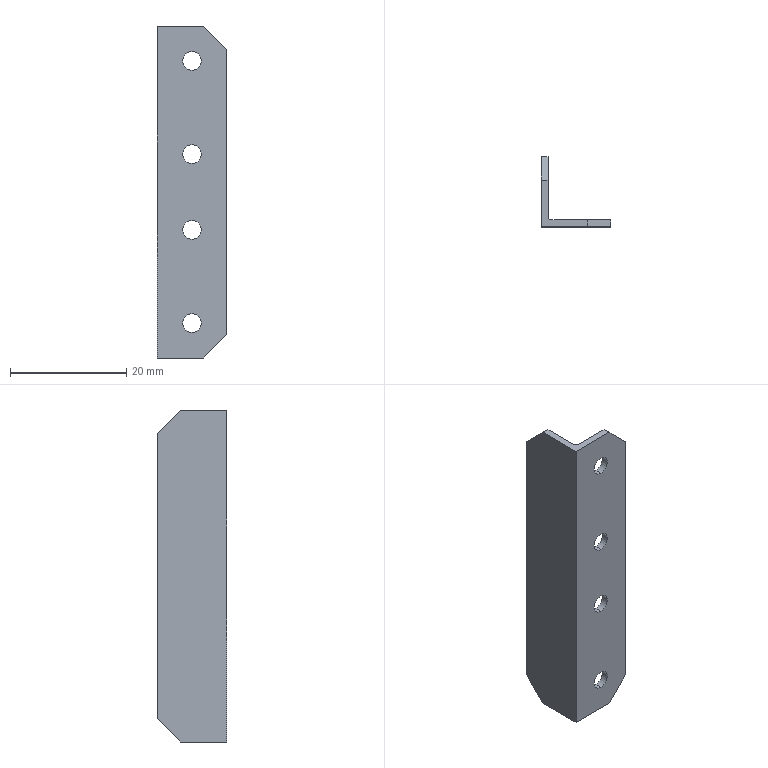Part | SolidWorks | features BaseBody 1 | 1 solid | 21 faces | box 12 x 12 x 57 mm | volume 1486 mm3 | plane 12 | cylinder 9 | commonest cylinder face diameters 3.2 x8 1 x1
STEP:
#1=CARTESIAN_POINT('',(6.,1.2,33.4));
#2=VERTEX_POINT('',#1);
#3=CARTESIAN_POINT('',(6.,1.2,36.6));
#4=VERTEX_POINT('',#3);
#5=CARTESIAN_POINT('',(6.,1.2,35.));
#6=DIRECTION('',(0.,1.,0.));
#7=DIRECTION('',(0.,0.,-1.));
#8=AXIS2_PLACEMENT_3D('',#5,#6,#7);
#9=CIRCLE('',#8,1.6);
#10=EDGE_CURVE('',#2,#4,#9,.T.);
#11=ORIENTED_EDGE('',*,*,#10,.T.);
#12=CARTESIAN_POINT('',(6.,0.,36.6));
#13=VERTEX_POINT('',#12);
#14=CARTESIAN_POINT('',(6.,1.2,36.6));
#15=DIRECTION('',(0.,-1.,0.));
#16=VECTOR('',#15,1000.);
#17=LINE('',#14,#16);
#18=EDGE_CURVE('',#4,#13,#17,.T.);
#19=ORIENTED_EDGE('',*,*,#18,.T.);
#20=CARTESIAN_POINT('',(6.,0.,33.4));
#21=VERTEX_POINT('',#20);
#22=CARTESIAN_POINT('',(6.,0.,35.));
#23=DIRECTION('',(0.,-1.,0.));
#24=DIRECTION('',(0.,0.,-1.));
#25=AXIS2_PLACEMENT_3D('',#22,#23,#24);
#26=CIRCLE('',#25,1.6);
#27=EDGE_CURVE('',#13,#21,#26,.T.);
#28=ORIENTED_EDGE('',*,*,#27,.T.);
#29=CARTESIAN_POINT('',(6.,1.2,33.4));
#30=DIRECTION('',(0.,-1.,0.));
#31=VECTOR('',#30,1000.);
#32=LINE('',#29,#31);
#33=EDGE_CURVE('',#2,#21,#32,.T.);
#34=ORIENTED_EDGE('',*,*,#33,.F.);
#35=EDGE_LOOP('',(#11,#19,#28,#34));
#36=FACE_OUTER_BOUND('',#35,.T.);
#37=CARTESIAN_POINT('',(6.,1.2,35.));
#38=DIRECTION('',(0.,-1.,0.));
#39=DIRECTION('',(0.,0.,-1.));
#40=AXIS2_PLACEMENT_3D('',#37,#38,#39);
#41=CYLINDRICAL_SURFACE('',#40,1.6);
#42=ADVANCED_FACE('',(#36),#41,.F.);
#43=CARTESIAN_POINT('',(6.,1.2,4.4));
#44=VERTEX_POINT('',#43);
#45=CARTESIAN_POINT('',(6.,1.2,7.6));
#46=VERTEX_POINT('',#45);
#47=CARTESIAN_POINT('',(6.,1.2,6.));
#48=DIRECTION('',(0.,1.,0.));
#49=DIRECTION('',(0.,0.,-1.));
#50=AXIS2_PLACEMENT_3D('',#47,#48,#49);
#51=CIRCLE('',#50,1.6);
#52=EDGE_CURVE('',#44,#46,#51,.T.);
#53=ORIENTED_EDGE('',*,*,#52,.T.);
#54=CARTESIAN_POINT('',(6.,0.,7.6));
#55=VERTEX_POINT('',#54);
#56=CARTESIAN_POINT('',(6.,1.2,7.6));
#57=DIRECTION('',(0.,-1.,0.));
#58=VECTOR('',#57,1000.);
#59=LINE('',#56,#58);
#60=EDGE_CURVE('',#46,#55,#59,.T.);
#61=ORIENTED_EDGE('',*,*,#60,.T.);
#62=CARTESIAN_POINT('',(6.,0.,4.4));
#63=VERTEX_POINT('',#62);
#64=CARTESIAN_POINT('',(6.,0.,6.));
#65=DIRECTION('',(0.,-1.,0.));
#66=DIRECTION('',(0.,0.,-1.));
#67=AXIS2_PLACEMENT_3D('',#64,#65,#66);
#68=CIRCLE('',#67,1.6);
#69=EDGE_CURVE('',#55,#63,#68,.T.);
#70=ORIENTED_EDGE('',*,*,#69,.T.);
#71=CARTESIAN_POINT('',(6.,1.2,4.4));
#72=DIRECTION('',(0.,-1.,0.));
#73=VECTOR('',#72,1000.);
#74=LINE('',#71,#73);
#75=EDGE_CURVE('',#44,#63,#74,.T.);
#76=ORIENTED_EDGE('',*,*,#75,.F.);
#77=EDGE_LOOP('',(#53,#61,#70,#76));
#78=FACE_OUTER_BOUND('',#77,.T.);
#79=CARTESIAN_POINT('',(6.,1.2,6.));
#80=DIRECTION('',(0.,-1.,0.));
#81=DIRECTION('',(0.,0.,-1.));
#82=AXIS2_PLACEMENT_3D('',#79,#80,#81);
#83=CYLINDRICAL_SURFACE('',#82,1.6);
#84=ADVANCED_FACE('',(#78),#83,.F.);
#85=CARTESIAN_POINT('',(6.,1.2,49.4));
#86=VERTEX_POINT('',#85);
#87=CARTESIAN_POINT('',(6.,1.2,52.6));
#88=VERTEX_POINT('',#87);
#89=CARTESIAN_POINT('',(6.,1.2,51.));
#90=DIRECTION('',(0.,1.,0.));
#91=DIRECTION('',(0.,0.,-1.));
#92=AXIS2_PLACEMENT_3D('',#89,#90,#91);
#93=CIRCLE('',#92,1.6);
#94=EDGE_CURVE('',#86,#88,#93,.T.);
#95=ORIENTED_EDGE('',*,*,#94,.T.);
#96=CARTESIAN_POINT('',(6.,0.,52.6));
#97=VERTEX_POINT('',#96);
#98=CARTESIAN_POINT('',(6.,1.2,52.6));
#99=DIRECTION('',(0.,-1.,0.));
#100=VECTOR('',#99,1000.);
#101=LINE('',#98,#100);
#102=EDGE_CURVE('',#88,#97,#101,.T.);
#103=ORIENTED_EDGE('',*,*,#102,.T.);
#104=CARTESIAN_POINT('',(6.,0.,49.4));
#105=VERTEX_POINT('',#104);
#106=CARTESIAN_POINT('',(6.,0.,51.));
#107=DIRECTION('',(0.,-1.,0.));
#108=DIRECTION('',(0.,0.,-1.));
#109=AXIS2_PLACEMENT_3D('',#106,#107,#108);
#110=CIRCLE('',#109,1.6);
#111=EDGE_CURVE('',#97,#105,#110,.T.);
#112=ORIENTED_EDGE('',*,*,#111,.T.);
#113=CARTESIAN_POINT('',(6.,1.2,49.4));
#114=DIRECTION('',(0.,-1.,0.));
#115=VECTOR('',#114,1000.);
#116=LINE('',#113,#115);
#117=EDGE_CURVE('',#86,#105,#116,.T.);
#118=ORIENTED_EDGE('',*,*,#117,.F.);
#119=EDGE_LOOP('',(#95,#103,#112,#118));
#120=FACE_OUTER_BOUND('',#119,.T.);
#121=CARTESIAN_POINT('',(6.,1.2,51.));
#122=DIRECTION('',(0.,-1.,0.));
#123=DIRECTION('',(0.,0.,-1.));
#124=AXIS2_PLACEMENT_3D('',#121,#122,#123);
#125=CYLINDRICAL_SURFACE('',#124,1.6);
#126=ADVANCED_FACE('',(#120),#125,.F.);
#127=CARTESIAN_POINT('',(6.,1.2,20.4));
#128=VERTEX_POINT('',#127);
#129=CARTESIAN_POINT('',(6.,1.2,23.6));
#130=VERTEX_POINT('',#129);
#131=CARTESIAN_POINT('',(6.,1.2,22.));
#132=DIRECTION('',(0.,1.,0.));
#133=DIRECTION('',(0.,0.,-1.));
#134=AXIS2_PLACEMENT_3D('',#131,#132,#133);
#135=CIRCLE('',#134,1.6);
#136=EDGE_CURVE('',#128,#130,#135,.T.);
#137=ORIENTED_EDGE('',*,*,#136,.T.);
#138=CARTESIAN_POINT('',(6.,0.,23.6));
#139=VERTEX_POINT('',#138);
#140=CARTESIAN_POINT('',(6.,1.2,23.6));
#141=DIRECTION('',(0.,-1.,0.));
#142=VECTOR('',#141,1000.);
#143=LINE('',#140,#142);
#144=EDGE_CURVE('',#130,#139,#143,.T.);
#145=ORIENTED_EDGE('',*,*,#144,.T.);
#146=CARTESIAN_POINT('',(6.,0.,20.4));
#147=VERTEX_POINT('',#146);
#148=CARTESIAN_POINT('',(6.,0.,22.));
#149=DIRECTION('',(0.,-1.,0.));
#150=DIRECTION('',(0.,0.,-1.));
#151=AXIS2_PLACEMENT_3D('',#148,#149,#150);
#152=CIRCLE('',#151,1.6);
#153=EDGE_CURVE('',#139,#147,#152,.T.);
#154=ORIENTED_EDGE('',*,*,#153,.T.);
#155=CARTESIAN_POINT('',(6.,1.2,20.4));
#156=DIRECTION('',(0.,-1.,0.));
#157=VECTOR('',#156,1000.);
#158=LINE('',#155,#157);
#159=EDGE_CURVE('',#128,#147,#158,.T.);
#160=ORIENTED_EDGE('',*,*,#159,.F.);
#161=EDGE_LOOP('',(#137,#145,#154,#160));
#162=FACE_OUTER_BOUND('',#161,.T.);
#163=CARTESIAN_POINT('',(6.,1.2,22.));
#164=DIRECTION('',(0.,-1.,0.));
#165=DIRECTION('',(0.,0.,-1.));
#166=AXIS2_PLACEMENT_3D('',#163,#164,#165);
#167=CYLINDRICAL_SURFACE('',#166,1.6);
#168=ADVANCED_FACE('',(#162),#167,.F.);
#169=ORIENTED_EDGE('',*,*,#18,.F.);
#170=CARTESIAN_POINT('',(6.,1.2,35.));
#171=DIRECTION('',(0.,1.,0.));
#172=DIRECTION('',(0.,0.,-1.));
#173=AXIS2_PLACEMENT_3D('',#170,#171,#172);
#174=CIRCLE('',#173,1.6);
#175=EDGE_CURVE('',#4,#2,#174,.T.);
#176=ORIENTED_EDGE('',*,*,#175,.T.);
#177=ORIENTED_EDGE('',*,*,#33,.T.);
#178=CARTESIAN_POINT('',(6.,0.,35.));
#179=DIRECTION('',(0.,-1.,0.));
#180=DIRECTION('',(0.,0.,-1.));
#181=AXIS2_PLACEMENT_3D('',#178,#179,#180);
#182=CIRCLE('',#181,1.6);
#183=EDGE_CURVE('',#21,#13,#182,.T.);
#184=ORIENTED_EDGE('',*,*,#183,.T.);
#185=EDGE_LOOP('',(#169,#176,#177,#184));
#186=FACE_OUTER_BOUND('',#185,.T.);
#187=CARTESIAN_POINT('',(6.,1.2,35.));
#188=DIRECTION('',(0.,-1.,0.));
#189=DIRECTION('',(0.,0.,-1.));
#190=AXIS2_PLACEMENT_3D('',#187,#188,#189);
#191=CYLINDRICAL_SURFACE('',#190,1.6);
#192=ADVANCED_FACE('',(#186),#191,.F.);
#193=CARTESIAN_POINT('',(6.,0.,6.));
#194=DIRECTION('',(0.,-1.,0.));
#195=DIRECTION('',(0.,0.,-1.));
#196=AXIS2_PLACEMENT_3D('',#193,#194,#195);
#197=CIRCLE('',#196,1.6);
#198=EDGE_CURVE('',#63,#55,#197,.T.);
#199=ORIENTED_EDGE('',*,*,#198,.F.);
#200=ORIENTED_EDGE('',*,*,#69,.F.);
#201=EDGE_LOOP('',(#199,#200));
#202=FACE_BOUND('',#201,.T.);
#203=CARTESIAN_POINT('',(6.,0.,51.));
#204=DIRECTION('',(0.,-1.,0.));
#205=DIRECTION('',(0.,0.,-1.));
#206=AXIS2_PLACEMENT_3D('',#203,#204,#205);
#207=CIRCLE('',#206,1.6);
#208=EDGE_CURVE('',#105,#97,#207,.T.);
#209=ORIENTED_EDGE('',*,*,#208,.F.);
#210=ORIENTED_EDGE('',*,*,#111,.F.);
#211=EDGE_LOOP('',(#209,#210));
#212=FACE_BOUND('',#211,.T.);
#213=CARTESIAN_POINT('',(6.,0.,22.));
#214=DIRECTION('',(0.,-1.,0.));
#215=DIRECTION('',(0.,0.,-1.));
#216=AXIS2_PLACEMENT_3D('',#213,#214,#215);
#217=CIRCLE('',#216,1.6);
#218=EDGE_CURVE('',#147,#139,#217,.T.);
#219=ORIENTED_EDGE('',*,*,#218,.F.);
#220=ORIENTED_EDGE('',*,*,#153,.F.);
#221=EDGE_LOOP('',(#219,#220));
#222=FACE_BOUND('',#221,.T.);
#223=ORIENTED_EDGE('',*,*,#183,.F.);
#224=ORIENTED_EDGE('',*,*,#27,.F.);
#225=EDGE_LOOP('',(#223,#224));
#226=FACE_BOUND('',#225,.T.);
#227=CARTESIAN_POINT('',(8.,0.,57.));
#228=VERTEX_POINT('',#227);
#229=CARTESIAN_POINT('',(12.,0.,53.));
#230=VERTEX_POINT('',#229);
#231=CARTESIAN_POINT('',(8.,0.,57.));
#232=DIRECTION('',(0.7071,0.,-0.7071));
#233=VECTOR('',#232,1000.);
#234=LINE('',#231,#233);
#235=EDGE_CURVE('',#228,#230,#234,.T.);
#236=ORIENTED_EDGE('',*,*,#235,.F.);
#237=CARTESIAN_POINT('',(0.,0.,57.));
#238=VERTEX_POINT('',#237);
#239=CARTESIAN_POINT('',(6.,0.,57.));
#240=DIRECTION('',(1.,0.,0.));
#241=VECTOR('',#240,1000.);
#242=LINE('',#239,#241);
#243=EDGE_CURVE('',#238,#228,#242,.T.);
#244=ORIENTED_EDGE('',*,*,#243,.F.);
#245=CARTESIAN_POINT('',(0.,0.,0.));
#246=VERTEX_POINT('',#245);
#247=CARTESIAN_POINT('',(0.,0.,28.5));
#248=DIRECTION('',(0.,0.,1.));
#249=VECTOR('',#248,1000.);
#250=LINE('',#247,#249);
#251=EDGE_CURVE('',#246,#238,#250,.T.);
#252=ORIENTED_EDGE('',*,*,#251,.F.);
#253=CARTESIAN_POINT('',(8.,0.,0.));
#254=VERTEX_POINT('',#253);
#255=CARTESIAN_POINT('',(6.,0.,0.));
#256=DIRECTION('',(-1.,0.,0.));
#257=VECTOR('',#256,1000.);
#258=LINE('',#255,#257);
#259=EDGE_CURVE('',#254,#246,#258,.T.);
#260=ORIENTED_EDGE('',*,*,#259,.F.);
#261=CARTESIAN_POINT('',(12.,0.,4.));
#262=VERTEX_POINT('',#261);
#263=CARTESIAN_POINT('',(8.,0.,0.));
#264=DIRECTION('',(-0.7071,0.,-0.7071));
#265=VECTOR('',#264,1000.);
#266=LINE('',#263,#265);
#267=EDGE_CURVE('',#262,#254,#266,.T.);
#268=ORIENTED_EDGE('',*,*,#267,.F.);
#269=CARTESIAN_POINT('',(12.,0.,28.5));
#270=DIRECTION('',(0.,0.,-1.));
#271=VECTOR('',#270,1000.);
#272=LINE('',#269,#271);
#273=EDGE_CURVE('',#230,#262,#272,.T.);
#274=ORIENTED_EDGE('',*,*,#273,.F.);
#275=EDGE_LOOP('',(#236,#244,#252,#260,#268,#274));
#276=FACE_OUTER_BOUND('',#275,.T.);
#277=CARTESIAN_POINT('',(0.,0.,0.));
#278=DIRECTION('',(0.,1.,0.));
#279=DIRECTION('',(0.,0.,1.));
#280=AXIS2_PLACEMENT_3D('',#277,#278,#279);
#281=PLANE('',#280);
#282=ADVANCED_FACE('',(#202,#212,#222,#226,#276),#281,.F.);
#283=ORIENTED_EDGE('',*,*,#52,.F.);
#284=CARTESIAN_POINT('',(6.,1.2,6.));
#285=DIRECTION('',(0.,1.,0.));
#286=DIRECTION('',(0.,0.,-1.));
#287=AXIS2_PLACEMENT_3D('',#284,#285,#286);
#288=CIRCLE('',#287,1.6);
#289=EDGE_CURVE('',#46,#44,#288,.T.);
#290=ORIENTED_EDGE('',*,*,#289,.F.);
#291=EDGE_LOOP('',(#283,#290));
#292=FACE_BOUND('',#291,.T.);
#293=ORIENTED_EDGE('',*,*,#94,.F.);
#294=CARTESIAN_POINT('',(6.,1.2,51.));
#295=DIRECTION('',(0.,1.,0.));
#296=DIRECTION('',(0.,0.,-1.));
#297=AXIS2_PLACEMENT_3D('',#294,#295,#296);
#298=CIRCLE('',#297,1.6);
#299=EDGE_CURVE('',#88,#86,#298,.T.);
#300=ORIENTED_EDGE('',*,*,#299,.F.);
#301=EDGE_LOOP('',(#293,#300));
#302=FACE_BOUND('',#301,.T.);
#303=ORIENTED_EDGE('',*,*,#136,.F.);
#304=CARTESIAN_POINT('',(6.,1.2,22.));
#305=DIRECTION('',(0.,1.,0.));
#306=DIRECTION('',(0.,0.,-1.));
#307=AXIS2_PLACEMENT_3D('',#304,#305,#306);
#308=CIRCLE('',#307,1.6);
#309=EDGE_CURVE('',#130,#128,#308,.T.);
#310=ORIENTED_EDGE('',*,*,#309,.F.);
#311=EDGE_LOOP('',(#303,#310));
#312=FACE_BOUND('',#311,.T.);
#313=ORIENTED_EDGE('',*,*,#10,.F.);
#314=ORIENTED_EDGE('',*,*,#175,.F.);
#315=EDGE_LOOP('',(#313,#314));
#316=FACE_BOUND('',#315,.T.);
#317=CARTESIAN_POINT('',(12.,1.2,53.));
#318=VERTEX_POINT('',#317);
#319=CARTESIAN_POINT('',(8.,1.2,57.));
#320=VERTEX_POINT('',#319);
#321=CARTESIAN_POINT('',(8.,1.2,57.));
#322=DIRECTION('',(-0.7071,0.,0.7071));
#323=VECTOR('',#322,1000.);
#324=LINE('',#321,#323);
#325=EDGE_CURVE('',#318,#320,#324,.T.);
#326=ORIENTED_EDGE('',*,*,#325,.F.);
#327=CARTESIAN_POINT('',(12.,1.2,4.));
#328=VERTEX_POINT('',#327);
#329=CARTESIAN_POINT('',(12.,1.2,28.5));
#330=DIRECTION('',(0.,0.,1.));
#331=VECTOR('',#330,1000.);
#332=LINE('',#329,#331);
#333=EDGE_CURVE('',#328,#318,#332,.T.);
#334=ORIENTED_EDGE('',*,*,#333,.F.);
#335=CARTESIAN_POINT('',(8.,1.2,0.));
#336=VERTEX_POINT('',#335);
#337=CARTESIAN_POINT('',(8.,1.2,0.));
#338=DIRECTION('',(0.7071,0.,0.7071));
#339=VECTOR('',#338,1000.);
#340=LINE('',#337,#339);
#341=EDGE_CURVE('',#336,#328,#340,.T.);
#342=ORIENTED_EDGE('',*,*,#341,.F.);
#343=CARTESIAN_POINT('',(1.7,1.2,0.));
#344=VERTEX_POINT('',#343);
#345=CARTESIAN_POINT('',(6.85,1.2,0.));
#346=DIRECTION('',(1.,0.,0.));
#347=VECTOR('',#346,1000.);
#348=LINE('',#345,#347);
#349=EDGE_CURVE('',#344,#336,#348,.T.);
#350=ORIENTED_EDGE('',*,*,#349,.F.);
#351=CARTESIAN_POINT('',(1.7,1.2,57.));
#352=VERTEX_POINT('',#351);
#353=CARTESIAN_POINT('',(1.7,1.2,28.5));
#354=DIRECTION('',(0.,0.,-1.));
#355=VECTOR('',#354,1000.);
#356=LINE('',#353,#355);
#357=EDGE_CURVE('',#352,#344,#356,.T.);
#358=ORIENTED_EDGE('',*,*,#357,.F.);
#359=CARTESIAN_POINT('',(6.85,1.2,57.));
#360=DIRECTION('',(-1.,0.,0.));
#361=VECTOR('',#360,1000.);
#362=LINE('',#359,#361);
#363=EDGE_CURVE('',#320,#352,#362,.T.);
#364=ORIENTED_EDGE('',*,*,#363,.F.);
#365=EDGE_LOOP('',(#326,#334,#342,#350,#358,#364));
#366=FACE_OUTER_BOUND('',#365,.T.);
#367=CARTESIAN_POINT('',(1.7,1.2,57.));
#368=DIRECTION('',(0.,-1.,0.));
#369=DIRECTION('',(0.,0.,-1.));
#370=AXIS2_PLACEMENT_3D('',#367,#368,#369);
#371=PLANE('',#370);
#372=ADVANCED_FACE('',(#292,#302,#312,#316,#366),#371,.F.);
#373=ORIENTED_EDGE('',*,*,#60,.F.);
#374=ORIENTED_EDGE('',*,*,#289,.T.);
#375=ORIENTED_EDGE('',*,*,#75,.T.);
#376=ORIENTED_EDGE('',*,*,#198,.T.);
#377=EDGE_LOOP('',(#373,#374,#375,#376));
#378=FACE_OUTER_BOUND('',#377,.T.);
#379=CARTESIAN_POINT('',(6.,1.2,6.));
#380=DIRECTION('',(0.,-1.,0.));
#381=DIRECTION('',(0.,0.,-1.));
#382=AXIS2_PLACEMENT_3D('',#379,#380,#381);
#383=CYLINDRICAL_SURFACE('',#382,1.6);
#384=ADVANCED_FACE('',(#378),#383,.F.);
#385=ORIENTED_EDGE('',*,*,#102,.F.);
#386=ORIENTED_EDGE('',*,*,#299,.T.);
#387=ORIENTED_EDGE('',*,*,#117,.T.);
#388=ORIENTED_EDGE('',*,*,#208,.T.);
#389=EDGE_LOOP('',(#385,#386,#387,#388));
#390=FACE_OUTER_BOUND('',#389,.T.);
#391=CARTESIAN_POINT('',(6.,1.2,51.));
#392=DIRECTION('',(0.,-1.,0.));
#393=DIRECTION('',(0.,0.,-1.));
#394=AXIS2_PLACEMENT_3D('',#391,#392,#393);
#395=CYLINDRICAL_SURFACE('',#394,1.6);
#396=ADVANCED_FACE('',(#390),#395,.F.);
#397=ORIENTED_EDGE('',*,*,#144,.F.);
#398=ORIENTED_EDGE('',*,*,#309,.T.);
#399=ORIENTED_EDGE('',*,*,#159,.T.);
#400=ORIENTED_EDGE('',*,*,#218,.T.);
#401=EDGE_LOOP('',(#397,#398,#399,#400));
#402=FACE_OUTER_BOUND('',#401,.T.);
#403=CARTESIAN_POINT('',(6.,1.2,22.));
#404=DIRECTION('',(0.,-1.,0.));
#405=DIRECTION('',(0.,0.,-1.));
#406=AXIS2_PLACEMENT_3D('',#403,#404,#405);
#407=CYLINDRICAL_SURFACE('',#406,1.6);
#408=ADVANCED_FACE('',(#402),#407,.F.);
#409=CARTESIAN_POINT('',(12.,0.6,53.));
#410=DIRECTION('',(0.,1.,0.));
#411=VECTOR('',#410,1000.);
#412=LINE('',#409,#411);
#413=EDGE_CURVE('',#230,#318,#412,.T.);
#414=ORIENTED_EDGE('',*,*,#413,.F.);
#415=ORIENTED_EDGE('',*,*,#273,.T.);
#416=CARTESIAN_POINT('',(12.,0.6,4.));
#417=DIRECTION('',(0.,-1.,0.));
#418=VECTOR('',#417,1000.);
#419=LINE('',#416,#418);
#420=EDGE_CURVE('',#328,#262,#419,.T.);
#421=ORIENTED_EDGE('',*,*,#420,.F.);
#422=ORIENTED_EDGE('',*,*,#333,.T.);
#423=EDGE_LOOP('',(#414,#415,#421,#422));
#424=FACE_OUTER_BOUND('',#423,.T.);
#425=CARTESIAN_POINT('',(12.,0.,4.));
#426=DIRECTION('',(-1.,0.,0.));
#427=DIRECTION('',(0.,0.,1.));
#428=AXIS2_PLACEMENT_3D('',#425,#426,#427);
#429=PLANE('',#428);
#430=ADVANCED_FACE('',(#424),#429,.F.);
#431=ORIENTED_EDGE('',*,*,#325,.T.);
#432=CARTESIAN_POINT('',(8.,0.6,57.));
#433=DIRECTION('',(0.,-1.,0.));
#434=VECTOR('',#433,1000.);
#435=LINE('',#432,#434);
#436=EDGE_CURVE('',#320,#228,#435,.T.);
#437=ORIENTED_EDGE('',*,*,#436,.T.);
#438=ORIENTED_EDGE('',*,*,#235,.T.);
#439=ORIENTED_EDGE('',*,*,#413,.T.);
#440=EDGE_LOOP('',(#431,#437,#438,#439));
#441=FACE_OUTER_BOUND('',#440,.T.);
#442=CARTESIAN_POINT('',(8.,0.,57.));
#443=DIRECTION('',(0.7071,0.,0.7071));
#444=DIRECTION('',(0.7071,0.,-0.7071));
#445=AXIS2_PLACEMENT_3D('',#442,#443,#444);
#446=PLANE('',#445);
#447=ADVANCED_FACE('',(#441),#446,.T.);
#448=CARTESIAN_POINT('',(0.,8.,57.));
#449=VERTEX_POINT('',#448);
#450=CARTESIAN_POINT('',(1.2,8.,57.));
#451=VERTEX_POINT('',#450);
#452=CARTESIAN_POINT('',(0.6,8.,57.));
#453=DIRECTION('',(1.,0.,0.));
#454=VECTOR('',#453,1000.);
#455=LINE('',#452,#454);
#456=EDGE_CURVE('',#449,#451,#455,.T.);
#457=ORIENTED_EDGE('',*,*,#456,.F.);
#458=CARTESIAN_POINT('',(0.,4.,57.));
#459=DIRECTION('',(0.,-1.,0.));
#460=VECTOR('',#459,1000.);
#461=LINE('',#458,#460);
#462=EDGE_CURVE('',#449,#238,#461,.T.);
#463=ORIENTED_EDGE('',*,*,#462,.T.);
#464=ORIENTED_EDGE('',*,*,#243,.T.);
#465=ORIENTED_EDGE('',*,*,#436,.F.);
#466=ORIENTED_EDGE('',*,*,#363,.T.);
#467=CARTESIAN_POINT('',(1.2,1.7,57.));
#468=VERTEX_POINT('',#467);
#469=CARTESIAN_POINT('',(1.7,1.7,57.));
#470=DIRECTION('',(0.,0.,-1.));
#471=DIRECTION('',(0.,1.,0.));
#472=AXIS2_PLACEMENT_3D('',#469,#470,#471);
#473=CIRCLE('',#472,0.5);
#474=EDGE_CURVE('',#352,#468,#473,.T.);
#475=ORIENTED_EDGE('',*,*,#474,.T.);
#476=CARTESIAN_POINT('',(1.2,4.,57.));
#477=DIRECTION('',(0.,1.,0.));
#478=VECTOR('',#477,1000.);
#479=LINE('',#476,#478);
#480=EDGE_CURVE('',#468,#451,#479,.T.);
#481=ORIENTED_EDGE('',*,*,#480,.T.);
#482=EDGE_LOOP('',(#457,#463,#464,#465,#466,#475,#481));
#483=FACE_OUTER_BOUND('',#482,.T.);
#484=CARTESIAN_POINT('',(0.,0.,57.));
#485=DIRECTION('',(0.,0.,1.));
#486=DIRECTION('',(1.,0.,0.));
#487=AXIS2_PLACEMENT_3D('',#484,#485,#486);
#488=PLANE('',#487);
#489=ADVANCED_FACE('',(#483),#488,.T.);
#490=CARTESIAN_POINT('',(0.,12.,53.));
#491=VERTEX_POINT('',#490);
#492=CARTESIAN_POINT('',(0.,12.,53.));
#493=DIRECTION('',(0.,-0.7071,0.7071));
#494=VECTOR('',#493,1000.);
#495=LINE('',#492,#494);
#496=EDGE_CURVE('',#491,#449,#495,.T.);
#497=ORIENTED_EDGE('',*,*,#496,.F.);
#498=CARTESIAN_POINT('',(0.,12.,4.));
#499=VERTEX_POINT('',#498);
#500=CARTESIAN_POINT('',(0.,12.,28.5));
#501=DIRECTION('',(0.,0.,1.));
#502=VECTOR('',#501,1000.);
#503=LINE('',#500,#502);
#504=EDGE_CURVE('',#499,#491,#503,.T.);
#505=ORIENTED_EDGE('',*,*,#504,.F.);
#506=CARTESIAN_POINT('',(0.,8.,0.));
#507=VERTEX_POINT('',#506);
#508=CARTESIAN_POINT('',(0.,12.,4.));
#509=DIRECTION('',(0.,0.7071,0.7071));
#510=VECTOR('',#509,1000.);
#511=LINE('',#508,#510);
#512=EDGE_CURVE('',#507,#499,#511,.T.);
#513=ORIENTED_EDGE('',*,*,#512,.F.);
#514=CARTESIAN_POINT('',(0.,6.,0.));
#515=DIRECTION('',(0.,1.,0.));
#516=VECTOR('',#515,1000.);
#517=LINE('',#514,#516);
#518=EDGE_CURVE('',#246,#507,#517,.T.);
#519=ORIENTED_EDGE('',*,*,#518,.F.);
#520=ORIENTED_EDGE('',*,*,#251,.T.);
#521=ORIENTED_EDGE('',*,*,#462,.F.);
#522=EDGE_LOOP('',(#497,#505,#513,#519,#520,#521));
#523=FACE_OUTER_BOUND('',#522,.T.);
#524=CARTESIAN_POINT('',(0.,0.,0.));
#525=DIRECTION('',(1.,0.,0.));
#526=DIRECTION('',(0.,1.,0.));
#527=AXIS2_PLACEMENT_3D('',#524,#525,#526);
#528=PLANE('',#527);
#529=ADVANCED_FACE('',(#523),#528,.F.);
#530=CARTESIAN_POINT('',(8.,4.,0.));
#531=DIRECTION('',(0.,1.,0.));
#532=VECTOR('',#531,1000.);
#533=LINE('',#530,#532);
#534=EDGE_CURVE('',#254,#336,#533,.T.);
#535=ORIENTED_EDGE('',*,*,#534,.F.);
#536=ORIENTED_EDGE('',*,*,#259,.T.);
#537=ORIENTED_EDGE('',*,*,#518,.T.);
#538=CARTESIAN_POINT('',(1.2,8.,0.));
#539=VERTEX_POINT('',#538);
#540=CARTESIAN_POINT('',(4.,8.,0.));
#541=DIRECTION('',(-1.,0.,0.));
#542=VECTOR('',#541,1000.);
#543=LINE('',#540,#542);
#544=EDGE_CURVE('',#539,#507,#543,.T.);
#545=ORIENTED_EDGE('',*,*,#544,.F.);
#546=CARTESIAN_POINT('',(1.2,1.7,0.));
#547=VERTEX_POINT('',#546);
#548=CARTESIAN_POINT('',(1.2,4.,0.));
#549=DIRECTION('',(0.,1.,0.));
#550=VECTOR('',#549,1000.);
#551=LINE('',#548,#550);
#552=EDGE_CURVE('',#547,#539,#551,.T.);
#553=ORIENTED_EDGE('',*,*,#552,.F.);
#554=CARTESIAN_POINT('',(1.7,1.7,0.));
#555=DIRECTION('',(0.,0.,-1.));
#556=DIRECTION('',(0.,1.,0.));
#557=AXIS2_PLACEMENT_3D('',#554,#555,#556);
#558=CIRCLE('',#557,0.5);
#559=EDGE_CURVE('',#344,#547,#558,.T.);
#560=ORIENTED_EDGE('',*,*,#559,.F.);
#561=ORIENTED_EDGE('',*,*,#349,.T.);
#562=EDGE_LOOP('',(#535,#536,#537,#545,#553,#560,#561));
#563=FACE_OUTER_BOUND('',#562,.T.);
#564=CARTESIAN_POINT('',(0.,0.,0.));
#565=DIRECTION('',(0.,0.,1.));
#566=DIRECTION('',(1.,0.,0.));
#567=AXIS2_PLACEMENT_3D('',#564,#565,#566);
#568=PLANE('',#567);
#569=ADVANCED_FACE('',(#563),#568,.F.);
#570=ORIENTED_EDGE('',*,*,#534,.T.);
#571=ORIENTED_EDGE('',*,*,#341,.T.);
#572=ORIENTED_EDGE('',*,*,#420,.T.);
#573=ORIENTED_EDGE('',*,*,#267,.T.);
#574=EDGE_LOOP('',(#570,#571,#572,#573));
#575=FACE_OUTER_BOUND('',#574,.T.);
#576=CARTESIAN_POINT('',(8.,0.,0.));
#577=DIRECTION('',(-0.7071,0.,0.7071));
#578=DIRECTION('',(0.7071,0.,0.7071));
#579=AXIS2_PLACEMENT_3D('',#576,#577,#578);
#580=PLANE('',#579);
#581=ADVANCED_FACE('',(#575),#580,.F.);
#582=ORIENTED_EDGE('',*,*,#474,.F.);
#583=ORIENTED_EDGE('',*,*,#357,.T.);
#584=ORIENTED_EDGE('',*,*,#559,.T.);
#585=CARTESIAN_POINT('',(1.2,1.7,28.5));
#586=DIRECTION('',(0.,0.,1.));
#587=VECTOR('',#586,1000.);
#588=LINE('',#585,#587);
#589=EDGE_CURVE('',#547,#468,#588,.T.);
#590=ORIENTED_EDGE('',*,*,#589,.T.);
#591=EDGE_LOOP('',(#582,#583,#584,#590));
#592=FACE_OUTER_BOUND('',#591,.T.);
#593=CARTESIAN_POINT('',(1.7,1.7,57.));
#594=DIRECTION('',(0.,0.,-1.));
#595=DIRECTION('',(0.,1.,0.));
#596=AXIS2_PLACEMENT_3D('',#593,#594,#595);
#597=CYLINDRICAL_SURFACE('',#596,0.5);
#598=ADVANCED_FACE('',(#592),#597,.F.);
#599=CARTESIAN_POINT('',(1.2,12.,53.));
#600=VERTEX_POINT('',#599);
#601=CARTESIAN_POINT('',(1.2,12.,53.));
#602=DIRECTION('',(0.,0.7071,-0.7071));
#603=VECTOR('',#602,1000.);
#604=LINE('',#601,#603);
#605=EDGE_CURVE('',#451,#600,#604,.T.);
#606=ORIENTED_EDGE('',*,*,#605,.F.);
#607=ORIENTED_EDGE('',*,*,#480,.F.);
#608=ORIENTED_EDGE('',*,*,#589,.F.);
#609=ORIENTED_EDGE('',*,*,#552,.T.);
#610=CARTESIAN_POINT('',(1.2,12.,4.));
#611=VERTEX_POINT('',#610);
#612=CARTESIAN_POINT('',(1.2,12.,4.));
#613=DIRECTION('',(0.,-0.7071,-0.7071));
#614=VECTOR('',#613,1000.);
#615=LINE('',#612,#614);
#616=EDGE_CURVE('',#611,#539,#615,.T.);
#617=ORIENTED_EDGE('',*,*,#616,.F.);
#618=CARTESIAN_POINT('',(1.2,12.,28.5));
#619=DIRECTION('',(0.,0.,-1.));
#620=VECTOR('',#619,1000.);
#621=LINE('',#618,#620);
#622=EDGE_CURVE('',#600,#611,#621,.T.);
#623=ORIENTED_EDGE('',*,*,#622,.F.);
#624=EDGE_LOOP('',(#606,#607,#608,#609,#617,#623));
#625=FACE_OUTER_BOUND('',#624,.T.);
#626=CARTESIAN_POINT('',(1.2,1.7,0.));
#627=DIRECTION('',(-1.,0.,0.));
#628=DIRECTION('',(0.,0.,1.));
#629=AXIS2_PLACEMENT_3D('',#626,#627,#628);
#630=PLANE('',#629);
#631=ADVANCED_FACE('',(#625),#630,.F.);
#632=ORIENTED_EDGE('',*,*,#496,.T.);
#633=ORIENTED_EDGE('',*,*,#456,.T.);
#634=ORIENTED_EDGE('',*,*,#605,.T.);
#635=CARTESIAN_POINT('',(0.6,12.,53.));
#636=DIRECTION('',(-1.,0.,0.));
#637=VECTOR('',#636,1000.);
#638=LINE('',#635,#637);
#639=EDGE_CURVE('',#600,#491,#638,.T.);
#640=ORIENTED_EDGE('',*,*,#639,.T.);
#641=EDGE_LOOP('',(#632,#633,#634,#640));
#642=FACE_OUTER_BOUND('',#641,.T.);
#643=CARTESIAN_POINT('',(0.,12.,53.));
#644=DIRECTION('',(0.,0.7071,0.7071));
#645=DIRECTION('',(0.,-0.7071,0.7071));
#646=AXIS2_PLACEMENT_3D('',#643,#644,#645);
#647=PLANE('',#646);
#648=ADVANCED_FACE('',(#642),#647,.T.);
#649=ORIENTED_EDGE('',*,*,#639,.F.);
#650=ORIENTED_EDGE('',*,*,#622,.T.);
#651=CARTESIAN_POINT('',(0.6,12.,4.));
#652=DIRECTION('',(1.,0.,0.));
#653=VECTOR('',#652,1000.);
#654=LINE('',#651,#653);
#655=EDGE_CURVE('',#499,#611,#654,.T.);
#656=ORIENTED_EDGE('',*,*,#655,.F.);
#657=ORIENTED_EDGE('',*,*,#504,.T.);
#658=EDGE_LOOP('',(#649,#650,#656,#657));
#659=FACE_OUTER_BOUND('',#658,.T.);
#660=CARTESIAN_POINT('',(0.,12.,53.));
#661=DIRECTION('',(0.,-1.,0.));
#662=DIRECTION('',(0.,0.,-1.));
#663=AXIS2_PLACEMENT_3D('',#660,#661,#662);
#664=PLANE('',#663);
#665=ADVANCED_FACE('',(#659),#664,.F.);
#666=ORIENTED_EDGE('',*,*,#544,.T.);
#667=ORIENTED_EDGE('',*,*,#512,.T.);
#668=ORIENTED_EDGE('',*,*,#655,.T.);
#669=ORIENTED_EDGE('',*,*,#616,.T.);
#670=EDGE_LOOP('',(#666,#667,#668,#669));
#671=FACE_OUTER_BOUND('',#670,.T.);
#672=CARTESIAN_POINT('',(0.,12.,4.));
#673=DIRECTION('',(0.,-0.7071,0.7071));
#674=DIRECTION('',(0.,-0.7071,-0.7071));
#675=AXIS2_PLACEMENT_3D('',#672,#673,#674);
#676=PLANE('',#675);
#677=ADVANCED_FACE('',(#671),#676,.F.);
#678=CLOSED_SHELL('',(#42,#84,#126,#168,#192,#282,#372,#384,#396,#408,#430,#447,#489,#529,#569,#581,#598,#631,#648,#665,#677));
#679=MANIFOLD_SOLID_BREP('',#678);
#680=CARTESIAN_POINT('',(0.,0.,0.));
#681=DIRECTION('',(0.,0.,1.));
#682=DIRECTION('',(1.,0.,0.));
#683=AXIS2_PLACEMENT_3D('',#680,#681,#682);
#684=(LENGTH_UNIT()NAMED_UNIT(*)SI_UNIT(.MILLI.,.METRE.));
#685=UNCERTAINTY_MEASURE_WITH_UNIT(LENGTH_MEASURE(0.00001),#684,'','');
#686=(NAMED_UNIT(*)PLANE_ANGLE_UNIT()SI_UNIT($,.RADIAN.));
#687=(NAMED_UNIT(*)SI_UNIT($,.STERADIAN.)SOLID_ANGLE_UNIT());
#688=(GEOMETRIC_REPRESENTATION_CONTEXT(3)GLOBAL_UNCERTAINTY_ASSIGNED_CONTEXT((#685))GLOBAL_UNIT_ASSIGNED_CONTEXT((#684,#686,#687))REPRESENTATION_CONTEXT('',''));
#689=ADVANCED_BREP_SHAPE_REPRESENTATION('',(#679,#683),#688);